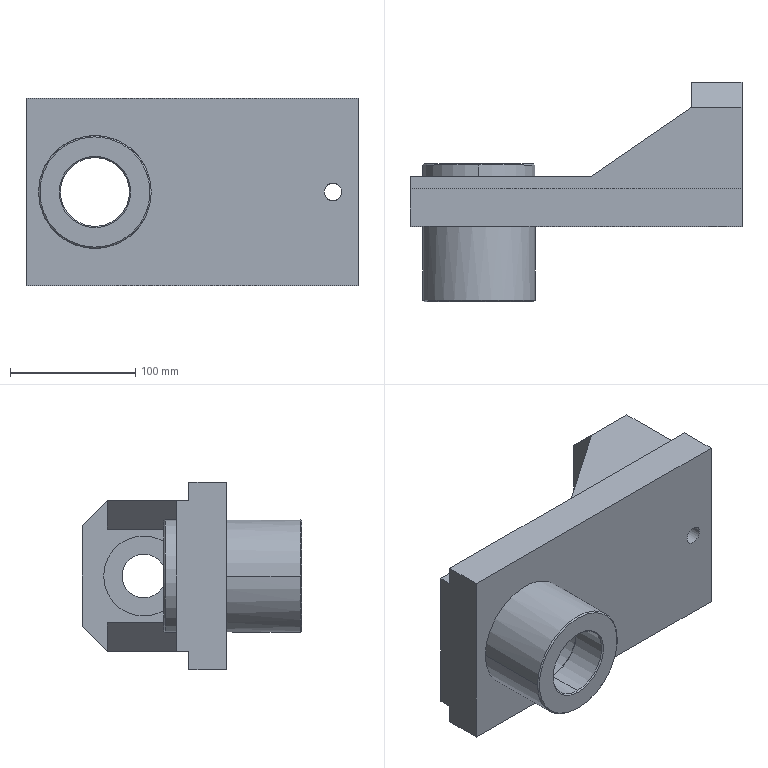Part | SolidWorks | features ICE 8, Chamfer 2, 3DProfileFeature 1, Extrusion 1, HoleWzd 1, RevCut 1 | 1 solid | 55 faces | box 265 x 175 x 150 mm | volume 1974640 mm3 | plane 25 | cylinder 18 | cone 12 | commonest cylinder face diameters 14 x4 90 x4 10 x2 35 x2 55 x2 56 x2